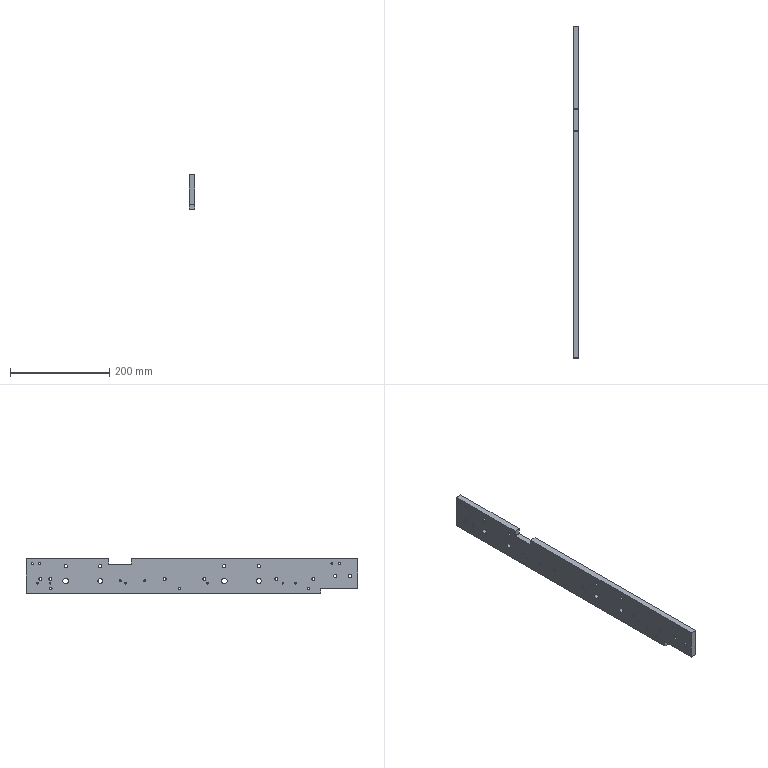Part | NX | features 5003_236_Mounting plate 2 | 1 solid | 57 faces | box 12 x 670 x 70 mm | volume 536912 mm3 | cylinder 35 | plane 16 | cone 6 | commonest cylinder face diameters 4.917 x9 3.3 x6 4.2 x6 10 x6 6.647 x4 2 x2